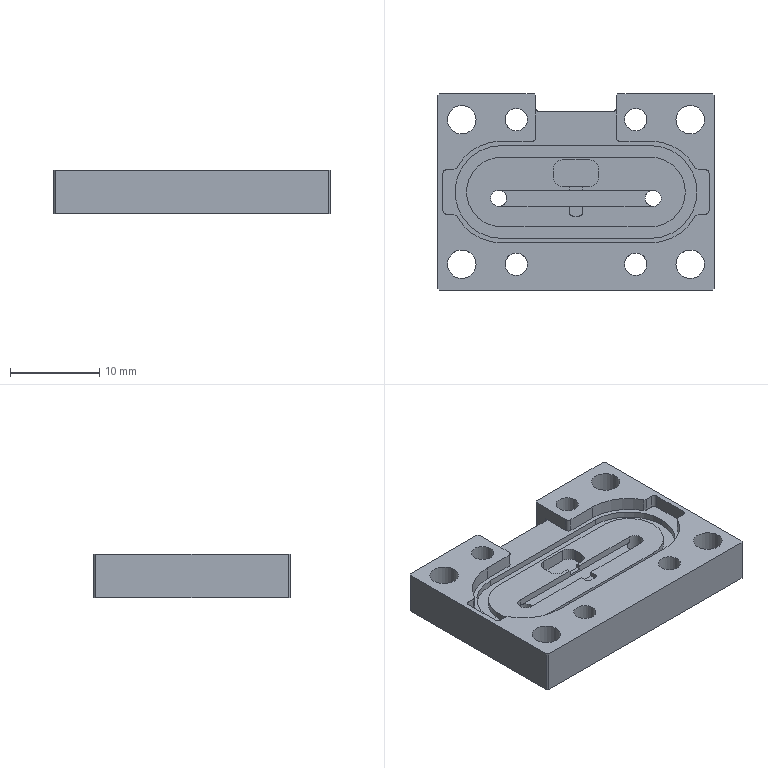NC program | NX | posted with a generic post | part box 31 x 22 x 4.9 mm
Lines 5425 to 7598 of 7945, first 1786 of 2168 lines:
(PLANAR_MILL_4_COPY_1 , TOOL : D0.8)
N10716 T10 M6
N10718 G54
N10720 G17 G0 G90 X-12.458 Y2.063 S3500 M3
N10722 G43 Z20. H10
N10724 Z0.14
N10726 G94 G1 Z-0.06 F200.
N10728 G41 X-12.493 Y2.157 D10
N10730 G3 X-13.18 Y2.327 R0.5
N10732 G1 X-13.463 Y2.157
N10734 G2 X-13.669 Y2.1 R0.4
N10736 G1 X-14.5
N10738 Y-2.1
N10740 X-13.669
N10742 G2 X-13.463 Y-2.157 R0.4
N10744 G1 X-13.18 Y-2.327
N10746 G3 X-12.493 Y-2.157 R0.5
N10748 G40
N10750 G1 X-12.458 Y-2.063
N10752 Z0.14
N10754 G0 Y2.063 Z0.08
N10756 G1 Z-0.12
N10758 G41 X-12.493 Y2.157
N10760 G3 X-13.18 Y2.327 R0.5
N10762 G1 X-13.463 Y2.157
N10764 G2 X-13.669 Y2.1 R0.4
N10766 G1 X-14.5
N10768 Y-2.1
N10770 X-13.669
N10772 G2 X-13.463 Y-2.157 R0.4
N10774 G1 X-13.18 Y-2.327
N10776 G3 X-12.493 Y-2.157 R0.5
N10778 G40
N10780 G1 X-12.458 Y-2.063
N10782 Z0.08
N10784 G0 Y2.063 Z0.02
N10786 G1 Z-0.18
N10788 G41 X-12.493 Y2.157
N10790 G3 X-13.18 Y2.327 R0.5
N10792 G1 X-13.463 Y2.157
N10794 G2 X-13.669 Y2.1 R0.4
N10796 G1 X-14.5
N10798 Y-2.1
N10800 X-13.669
N10802 G2 X-13.463 Y-2.157 R0.4
N10804 G1 X-13.18 Y-2.327
N10806 G3 X-12.493 Y-2.157 R0.5
N10808 G40
N10810 G1 X-12.458 Y-2.063
N10812 Z0.02
N10814 G0 Y2.063 Z-0.04
N10816 G1 Z-0.24
N10818 G41 X-12.493 Y2.157
N10820 G3 X-13.18 Y2.327 R0.5
N10822 G1 X-13.463 Y2.157
N10824 G2 X-13.669 Y2.1 R0.4
N10826 G1 X-14.5
N10828 Y-2.1
N10830 X-13.669
N10832 G2 X-13.463 Y-2.157 R0.4
N10834 G1 X-13.18 Y-2.327
N10836 G3 X-12.493 Y-2.157 R0.5
N10838 G40
N10840 G1 X-12.458 Y-2.063
N10842 Z-0.04
N10844 G0 Y2.063 Z-0.1
N10846 G1 Z-0.3
N10848 G41 X-12.493 Y2.157
N10850 G3 X-13.18 Y2.327 R0.5
N10852 G1 X-13.463 Y2.157
N10854 G2 X-13.669 Y2.1 R0.4
N10856 G1 X-14.5
N10858 Y-2.1
N10860 X-13.669
N10862 G2 X-13.463 Y-2.157 R0.4
N10864 G1 X-13.18 Y-2.327
N10866 G3 X-12.493 Y-2.157 R0.5
N10868 G40
N10870 G1 X-12.458 Y-2.063
N10872 Z-0.1
N10874 G0 Y2.063 Z-0.16
N10876 G1 Z-0.36
N10878 G41 X-12.493 Y2.157
N10880 G3 X-13.18 Y2.327 R0.5
N10882 G1 X-13.463 Y2.157
N10884 G2 X-13.669 Y2.1 R0.4
N10886 G1 X-14.5
N10888 Y-2.1
N10890 X-13.669
N10892 G2 X-13.463 Y-2.157 R0.4
N10894 G1 X-13.18 Y-2.327
N10896 G3 X-12.493 Y-2.157 R0.5
N10898 G40
N10900 G1 X-12.458 Y-2.063
N10902 Z-0.16
N10904 G0 Y2.063 Z-0.22
N10906 G1 Z-0.42
N10908 G41 X-12.493 Y2.157
N10910 G3 X-13.18 Y2.327 R0.5
N10912 G1 X-13.463 Y2.157
N10914 G2 X-13.669 Y2.1 R0.4
N10916 G1 X-14.5
N10918 Y-2.1
N10920 X-13.669
N10922 G2 X-13.463 Y-2.157 R0.4
N10924 G1 X-13.18 Y-2.327
N10926 G3 X-12.493 Y-2.157 R0.5
N10928 G40
N10930 G1 X-12.458 Y-2.063
N10932 Z-0.22
N10934 G0 Y2.063 Z-0.28
N10936 G1 Z-0.48
N10938 G41 X-12.493 Y2.157
N10940 G3 X-13.18 Y2.327 R0.5
N10942 G1 X-13.463 Y2.157
N10944 G2 X-13.669 Y2.1 R0.4
N10946 G1 X-14.5
N10948 Y-2.1
N10950 X-13.669
N10952 G2 X-13.463 Y-2.157 R0.4
N10954 G1 X-13.18 Y-2.327
N10956 G3 X-12.493 Y-2.157 R0.5
N10958 G40
N10960 G1 X-12.458 Y-2.063
N10962 Z-0.28
N10964 G0 Y2.063 Z-0.34
N10966 G1 Z-0.54
N10968 G41 X-12.493 Y2.157
N10970 G3 X-13.18 Y2.327 R0.5
N10972 G1 X-13.463 Y2.157
N10974 G2 X-13.669 Y2.1 R0.4
N10976 G1 X-14.5
N10978 Y-2.1
N10980 X-13.669
N10982 G2 X-13.463 Y-2.157 R0.4
N10984 G1 X-13.18 Y-2.327
N10986 G3 X-12.493 Y-2.157 R0.5
N10988 G40
N10990 G1 X-12.458 Y-2.063
N10992 Z-0.34
N10994 G0 Y2.063 Z-0.4
N10996 G1 Z-0.6
N10998 G41 X-12.493 Y2.157
N11000 G3 X-13.18 Y2.327 R0.5
N11002 G1 X-13.463 Y2.157
N11004 G2 X-13.669 Y2.1 R0.4
N11006 G1 X-14.5
N11008 Y-2.1
N11010 X-13.669
N11012 G2 X-13.463 Y-2.157 R0.4
N11014 G1 X-13.18 Y-2.327
N11016 G3 X-12.493 Y-2.157 R0.5
N11018 G40
N11020 G1 X-12.458 Y-2.063
N11022 Z-0.4
N11024 G0 Y2.063 Z-0.46
N11026 G1 Z-0.66
N11028 G41 X-12.493 Y2.157
N11030 G3 X-13.18 Y2.327 R0.5
N11032 G1 X-13.463 Y2.157
N11034 G2 X-13.669 Y2.1 R0.4
N11036 G1 X-14.5
N11038 Y-2.1
N11040 X-13.669
N11042 G2 X-13.463 Y-2.157 R0.4
N11044 G1 X-13.18 Y-2.327
N11046 G3 X-12.493 Y-2.157 R0.5
N11048 G40
N11050 G1 X-12.458 Y-2.063
N11052 Z-0.46
N11054 G0 Y2.063 Z-0.52
N11056 G1 Z-0.72
N11058 G41 X-12.493 Y2.157
N11060 G3 X-13.18 Y2.327 R0.5
N11062 G1 X-13.463 Y2.157
N11064 G2 X-13.669 Y2.1 R0.4
N11066 G1 X-14.5
N11068 Y-2.1
N11070 X-13.669
N11072 G2 X-13.463 Y-2.157 R0.4
N11074 G1 X-13.18 Y-2.327
N11076 G3 X-12.493 Y-2.157 R0.5
N11078 G40
N11080 G1 X-12.458 Y-2.063
N11082 Z-0.52
N11084 G0 Y2.063 Z-0.58
N11086 G1 Z-0.78
N11088 G41 X-12.493 Y2.157
N11090 G3 X-13.18 Y2.327 R0.5
N11092 G1 X-13.463 Y2.157
N11094 G2 X-13.669 Y2.1 R0.4
N11096 G1 X-14.5
N11098 Y-2.1
N11100 X-13.669
N11102 G2 X-13.463 Y-2.157 R0.4
N11104 G1 X-13.18 Y-2.327
N11106 G3 X-12.493 Y-2.157 R0.5
N11108 G40
N11110 G1 X-12.458 Y-2.063
N11112 Z-0.58
N11114 G0 Y2.063 Z-0.64
N11116 G1 Z-0.84
N11118 G41 X-12.493 Y2.157
N11120 G3 X-13.18 Y2.327 R0.5
N11122 G1 X-13.463 Y2.157
N11124 G2 X-13.669 Y2.1 R0.4
N11126 G1 X-14.5
N11128 Y-2.1
N11130 X-13.669
N11132 G2 X-13.463 Y-2.157 R0.4
N11134 G1 X-13.18 Y-2.327
N11136 G3 X-12.493 Y-2.157 R0.5
N11138 G40
N11140 G1 X-12.458 Y-2.063
N11142 Z-0.64
N11144 G0 Y2.063 Z-0.7
N11146 G1 Z-0.9
N11148 G41 X-12.493 Y2.157
N11150 G3 X-13.18 Y2.327 R0.5
N11152 G1 X-13.463 Y2.157
N11154 G2 X-13.669 Y2.1 R0.4
N11156 G1 X-14.5
N11158 Y-2.1
N11160 X-13.669
N11162 G2 X-13.463 Y-2.157 R0.4
N11164 G1 X-13.18 Y-2.327
N11166 G3 X-12.493 Y-2.157 R0.5
N11168 G40
N11170 G1 X-12.458 Y-2.063
N11172 Z-0.7
N11174 G0 Y2.063 Z-0.76
N11176 G1 Z-0.96
N11178 G41 X-12.493 Y2.157
N11180 G3 X-13.18 Y2.327 R0.5
N11182 G1 X-13.463 Y2.157
N11184 G2 X-13.669 Y2.1 R0.4
N11186 G1 X-14.5
N11188 Y-2.1
N11190 X-13.669
N11192 G2 X-13.463 Y-2.157 R0.4
N11194 G1 X-13.18 Y-2.327
N11196 G3 X-12.493 Y-2.157 R0.5
N11198 G40
N11200 G1 X-12.458 Y-2.063
N11202 Z-0.76
N11204 G0 Y2.063 Z-0.82
N11206 G1 Z-1.02
N11208 G41 X-12.493 Y2.157
N11210 G3 X-13.18 Y2.327 R0.5
N11212 G1 X-13.463 Y2.157
N11214 G2 X-13.669 Y2.1 R0.4
N11216 G1 X-14.5
N11218 Y-2.1
N11220 X-13.669
N11222 G2 X-13.463 Y-2.157 R0.4
N11224 G1 X-13.18 Y-2.327
N11226 G3 X-12.493 Y-2.157 R0.5
N11228 G40
N11230 G1 X-12.458 Y-2.063
N11232 Z-0.82
N11234 G0 Y2.063 Z-0.88
N11236 G1 Z-1.08
N11238 G41 X-12.493 Y2.157
N11240 G3 X-13.18 Y2.327 R0.5
N11242 G1 X-13.463 Y2.157
N11244 G2 X-13.669 Y2.1 R0.4
N11246 G1 X-14.5
N11248 Y-2.1
N11250 X-13.669
N11252 G2 X-13.463 Y-2.157 R0.4
N11254 G1 X-13.18 Y-2.327
N11256 G3 X-12.493 Y-2.157 R0.5
N11258 G40
N11260 G1 X-12.458 Y-2.063
N11262 Z-0.88
N11264 G0 Y2.063 Z-0.94
N11266 G1 Z-1.14
N11268 G41 X-12.493 Y2.157
N11270 G3 X-13.18 Y2.327 R0.5
N11272 G1 X-13.463 Y2.157
N11274 G2 X-13.669 Y2.1 R0.4
N11276 G1 X-14.5
N11278 Y-2.1
N11280 X-13.669
N11282 G2 X-13.463 Y-2.157 R0.4
N11284 G1 X-13.18 Y-2.327
N11286 G3 X-12.493 Y-2.157 R0.5
N11288 G40
N11290 G1 X-12.458 Y-2.063
N11292 Z-0.94
N11294 G0 Y2.063 Z-1.
N11296 G1 Z-1.2
N11298 G41 X-12.493 Y2.157
N11300 G3 X-13.18 Y2.327 R0.5
N11302 G1 X-13.463 Y2.157
N11304 G2 X-13.669 Y2.1 R0.4
N11306 G1 X-14.5
N11308 Y-2.1
N11310 X-13.669
N11312 G2 X-13.463 Y-2.157 R0.4
N11314 G1 X-13.18 Y-2.327
N11316 G3 X-12.493 Y-2.157 R0.5
N11318 G40
N11320 G1 X-12.458 Y-2.063
N11322 Z-1.
N11324 G0 Y2.063 Z-1.06
N11326 G1 Z-1.26
N11328 G41 X-12.493 Y2.157
N11330 G3 X-13.18 Y2.327 R0.5
N11332 G1 X-13.463 Y2.157
N11334 G2 X-13.669 Y2.1 R0.4
N11336 G1 X-14.5
N11338 Y-2.1
N11340 X-13.669
N11342 G2 X-13.463 Y-2.157 R0.4
N11344 G1 X-13.18 Y-2.327
N11346 G3 X-12.493 Y-2.157 R0.5
N11348 G40
N11350 G1 X-12.458 Y-2.063
N11352 Z-1.06
N11354 G0 Y2.063 Z-1.12
N11356 G1 Z-1.32
N11358 G41 X-12.493 Y2.157
N11360 G3 X-13.18 Y2.327 R0.5
N11362 G1 X-13.463 Y2.157
N11364 G2 X-13.669 Y2.1 R0.4
N11366 G1 X-14.5
N11368 Y-2.1
N11370 X-13.669
N11372 G2 X-13.463 Y-2.157 R0.4
N11374 G1 X-13.18 Y-2.327
N11376 G3 X-12.493 Y-2.157 R0.5
N11378 G40
N11380 G1 X-12.458 Y-2.063
N11382 Z-1.12
N11384 G0 Y2.063 Z-1.18
N11386 G1 Z-1.38
N11388 G41 X-12.493 Y2.157
N11390 G3 X-13.18 Y2.327 R0.5
N11392 G1 X-13.463 Y2.157
N11394 G2 X-13.669 Y2.1 R0.4
N11396 G1 X-14.5
N11398 Y-2.1
N11400 X-13.669
N11402 G2 X-13.463 Y-2.157 R0.4
N11404 G1 X-13.18 Y-2.327
N11406 G3 X-12.493 Y-2.157 R0.5
N11408 G40
N11410 G1 X-12.458 Y-2.063
N11412 Z-1.18
N11414 G0 Y2.063 Z-1.24
N11416 G1 Z-1.44
N11418 G41 X-12.493 Y2.157
N11420 G3 X-13.18 Y2.327 R0.5
N11422 G1 X-13.463 Y2.157
N11424 G2 X-13.669 Y2.1 R0.4
N11426 G1 X-14.5
N11428 Y-2.1
N11430 X-13.669
N11432 G2 X-13.463 Y-2.157 R0.4
N11434 G1 X-13.18 Y-2.327
N11436 G3 X-12.493 Y-2.157 R0.5
N11438 G40
N11440 G1 X-12.458 Y-2.063
N11442 Z-1.24
N11444 G0 Y2.063 Z-1.3
N11446 G1 Z-1.5
N11448 G41 X-12.493 Y2.157
N11450 G3 X-13.18 Y2.327 R0.5
N11452 G1 X-13.463 Y2.157
N11454 G2 X-13.669 Y2.1 R0.4
N11456 G1 X-14.5
N11458 Y-2.1
N11460 X-13.669
N11462 G2 X-13.463 Y-2.157 R0.4
N11464 G1 X-13.18 Y-2.327
N11466 G3 X-12.493 Y-2.157 R0.5
N11468 G40
N11470 G1 X-12.458 Y-2.063
N11472 Z-1.3
N11474 G0 Z3.
N11476 X12.458
N11478 Z0.14
N11480 G1 Z-0.06
N11482 G41 X12.493 Y-2.157
N11484 G3 X13.18 Y-2.327 R0.5
N11486 G1 X13.463 Y-2.157
N11488 G2 X13.669 Y-2.1 R0.4
N11490 G1 X14.5
N11492 Y2.1
N11494 X13.669
N11496 G2 X13.463 Y2.157 R0.4
N11498 G1 X13.18 Y2.327
N11500 G3 X12.493 Y2.157 R0.5
N11502 G40
N11504 G1 X12.458 Y2.063
N11506 Z0.14
N11508 G0 Y-2.063 Z0.08
N11510 G1 Z-0.12
N11512 G41 X12.493 Y-2.157
N11514 G3 X13.18 Y-2.327 R0.5
N11516 G1 X13.463 Y-2.157
N11518 G2 X13.669 Y-2.1 R0.4
N11520 G1 X14.5
N11522 Y2.1
N11524 X13.669
N11526 G2 X13.463 Y2.157 R0.4
N11528 G1 X13.18 Y2.327
N11530 G3 X12.493 Y2.157 R0.5
N11532 G40
N11534 G1 X12.458 Y2.063
N11536 Z0.08
N11538 G0 Y-2.063 Z0.02
N11540 G1 Z-0.18
N11542 G41 X12.493 Y-2.157
N11544 G3 X13.18 Y-2.327 R0.5
N11546 G1 X13.463 Y-2.157
N11548 G2 X13.669 Y-2.1 R0.4
N11550 G1 X14.5
N11552 Y2.1
N11554 X13.669
N11556 G2 X13.463 Y2.157 R0.4
N11558 G1 X13.18 Y2.327
N11560 G3 X12.493 Y2.157 R0.5
N11562 G40
N11564 G1 X12.458 Y2.063
N11566 Z0.02
N11568 G0 Y-2.063 Z-0.04
N11570 G1 Z-0.24
N11572 G41 X12.493 Y-2.157
N11574 G3 X13.18 Y-2.327 R0.5
N11576 G1 X13.463 Y-2.157
N11578 G2 X13.669 Y-2.1 R0.4
N11580 G1 X14.5
N11582 Y2.1
N11584 X13.669
N11586 G2 X13.463 Y2.157 R0.4
N11588 G1 X13.18 Y2.327
N11590 G3 X12.493 Y2.157 R0.5
N11592 G40
N11594 G1 X12.458 Y2.063
N11596 Z-0.04
N11598 G0 Y-2.063 Z-0.1
N11600 G1 Z-0.3
N11602 G41 X12.493 Y-2.157
N11604 G3 X13.18 Y-2.327 R0.5
N11606 G1 X13.463 Y-2.157
N11608 G2 X13.669 Y-2.1 R0.4
N11610 G1 X14.5
N11612 Y2.1
N11614 X13.669
N11616 G2 X13.463 Y2.157 R0.4
N11618 G1 X13.18 Y2.327
N11620 G3 X12.493 Y2.157 R0.5
N11622 G40
N11624 G1 X12.458 Y2.063
N11626 Z-0.1
N11628 G0 Y-2.063 Z-0.16
N11630 G1 Z-0.36
N11632 G41 X12.493 Y-2.157
N11634 G3 X13.18 Y-2.327 R0.5
N11636 G1 X13.463 Y-2.157
N11638 G2 X13.669 Y-2.1 R0.4
N11640 G1 X14.5
N11642 Y2.1
N11644 X13.669
N11646 G2 X13.463 Y2.157 R0.4
N11648 G1 X13.18 Y2.327
N11650 G3 X12.493 Y2.157 R0.5
N11652 G40
N11654 G1 X12.458 Y2.063
N11656 Z-0.16
N11658 G0 Y-2.063 Z-0.22
N11660 G1 Z-0.42
N11662 G41 X12.493 Y-2.157
N11664 G3 X13.18 Y-2.327 R0.5
N11666 G1 X13.463 Y-2.157
N11668 G2 X13.669 Y-2.1 R0.4
N11670 G1 X14.5
N11672 Y2.1
N11674 X13.669
N11676 G2 X13.463 Y2.157 R0.4
N11678 G1 X13.18 Y2.327
N11680 G3 X12.493 Y2.157 R0.5
N11682 G40
N11684 G1 X12.458 Y2.063
N11686 Z-0.22
N11688 G0 Y-2.063 Z-0.28
N11690 G1 Z-0.48
N11692 G41 X12.493 Y-2.157
N11694 G3 X13.18 Y-2.327 R0.5
N11696 G1 X13.463 Y-2.157
N11698 G2 X13.669 Y-2.1 R0.4
N11700 G1 X14.5
N11702 Y2.1
N11704 X13.669
N11706 G2 X13.463 Y2.157 R0.4
N11708 G1 X13.18 Y2.327
N11710 G3 X12.493 Y2.157 R0.5
N11712 G40
N11714 G1 X12.458 Y2.063
N11716 Z-0.28
N11718 G0 Y-2.063 Z-0.34
N11720 G1 Z-0.54
N11722 G41 X12.493 Y-2.157
N11724 G3 X13.18 Y-2.327 R0.5
N11726 G1 X13.463 Y-2.157
N11728 G2 X13.669 Y-2.1 R0.4
N11730 G1 X14.5
N11732 Y2.1
N11734 X13.669
N11736 G2 X13.463 Y2.157 R0.4
N11738 G1 X13.18 Y2.327
N11740 G3 X12.493 Y2.157 R0.5
N11742 G40
N11744 G1 X12.458 Y2.063
N11746 Z-0.34
N11748 G0 Y-2.063 Z-0.4
N11750 G1 Z-0.6
N11752 G41 X12.493 Y-2.157
N11754 G3 X13.18 Y-2.327 R0.5
N11756 G1 X13.463 Y-2.157
N11758 G2 X13.669 Y-2.1 R0.4
N11760 G1 X14.5
N11762 Y2.1
N11764 X13.669
N11766 G2 X13.463 Y2.157 R0.4
N11768 G1 X13.18 Y2.327
N11770 G3 X12.493 Y2.157 R0.5
N11772 G40
N11774 G1 X12.458 Y2.063
N11776 Z-0.4
N11778 G0 Y-2.063 Z-0.46
N11780 G1 Z-0.66
N11782 G41 X12.493 Y-2.157
N11784 G3 X13.18 Y-2.327 R0.5
N11786 G1 X13.463 Y-2.157
N11788 G2 X13.669 Y-2.1 R0.4
N11790 G1 X14.5
N11792 Y2.1
N11794 X13.669
N11796 G2 X13.463 Y2.157 R0.4
N11798 G1 X13.18 Y2.327
N11800 G3 X12.493 Y2.157 R0.5
N11802 G40
N11804 G1 X12.458 Y2.063
N11806 Z-0.46
N11808 G0 Y-2.063 Z-0.52
N11810 G1 Z-0.72
N11812 G41 X12.493 Y-2.157
N11814 G3 X13.18 Y-2.327 R0.5
N11816 G1 X13.463 Y-2.157
N11818 G2 X13.669 Y-2.1 R0.4
N11820 G1 X14.5
N11822 Y2.1
N11824 X13.669
N11826 G2 X13.463 Y2.157 R0.4
N11828 G1 X13.18 Y2.327
N11830 G3 X12.493 Y2.157 R0.5
N11832 G40
N11834 G1 X12.458 Y2.063
N11836 Z-0.52
N11838 G0 Y-2.063 Z-0.58
N11840 G1 Z-0.78
N11842 G41 X12.493 Y-2.157
N11844 G3 X13.18 Y-2.327 R0.5
N11846 G1 X13.463 Y-2.157
N11848 G2 X13.669 Y-2.1 R0.4
N11850 G1 X14.5
N11852 Y2.1
N11854 X13.669
N11856 G2 X13.463 Y2.157 R0.4
N11858 G1 X13.18 Y2.327
N11860 G3 X12.493 Y2.157 R0.5
N11862 G40
N11864 G1 X12.458 Y2.063
N11866 Z-0.58
N11868 G0 Y-2.063 Z-0.64
N11870 G1 Z-0.84
N11872 G41 X12.493 Y-2.157
N11874 G3 X13.18 Y-2.327 R0.5
N11876 G1 X13.463 Y-2.157
N11878 G2 X13.669 Y-2.1 R0.4
N11880 G1 X14.5
N11882 Y2.1
N11884 X13.669
N11886 G2 X13.463 Y2.157 R0.4
N11888 G1 X13.18 Y2.327
N11890 G3 X12.493 Y2.157 R0.5
N11892 G40
N11894 G1 X12.458 Y2.063
N11896 Z-0.64
N11898 G0 Y-2.063 Z-0.7
N11900 G1 Z-0.9
N11902 G41 X12.493 Y-2.157
N11904 G3 X13.18 Y-2.327 R0.5
N11906 G1 X13.463 Y-2.157
N11908 G2 X13.669 Y-2.1 R0.4
N11910 G1 X14.5
N11912 Y2.1
N11914 X13.669
N11916 G2 X13.463 Y2.157 R0.4
N11918 G1 X13.18 Y2.327
N11920 G3 X12.493 Y2.157 R0.5
N11922 G40
N11924 G1 X12.458 Y2.063
N11926 Z-0.7
N11928 G0 Y-2.063 Z-0.76
N11930 G1 Z-0.96
N11932 G41 X12.493 Y-2.157
N11934 G3 X13.18 Y-2.327 R0.5
N11936 G1 X13.463 Y-2.157
N11938 G2 X13.669 Y-2.1 R0.4
N11940 G1 X14.5
N11942 Y2.1
N11944 X13.669
N11946 G2 X13.463 Y2.157 R0.4
N11948 G1 X13.18 Y2.327
N11950 G3 X12.493 Y2.157 R0.5
N11952 G40
N11954 G1 X12.458 Y2.063
N11956 Z-0.76
N11958 G0 Y-2.063 Z-0.82
N11960 G1 Z-1.02
N11962 G41 X12.493 Y-2.157
N11964 G3 X13.18 Y-2.327 R0.5
N11966 G1 X13.463 Y-2.157
N11968 G2 X13.669 Y-2.1 R0.4
N11970 G1 X14.5
N11972 Y2.1
N11974 X13.669
N11976 G2 X13.463 Y2.157 R0.4
N11978 G1 X13.18 Y2.327
N11980 G3 X12.493 Y2.157 R0.5
N11982 G40
N11984 G1 X12.458 Y2.063
N11986 Z-0.82
N11988 G0 Y-2.063 Z-0.88
N11990 G1 Z-1.08
N11992 G41 X12.493 Y-2.157
N11994 G3 X13.18 Y-2.327 R0.5
N11996 G1 X13.463 Y-2.157
N11998 G2 X13.669 Y-2.1 R0.4
N12000 G1 X14.5
N12002 Y2.1
N12004 X13.669
N12006 G2 X13.463 Y2.157 R0.4
N12008 G1 X13.18 Y2.327
N12010 G3 X12.493 Y2.157 R0.5
N12012 G40
N12014 G1 X12.458 Y2.063
N12016 Z-0.88
N12018 G0 Y-2.063 Z-0.94
N12020 G1 Z-1.14
N12022 G41 X12.493 Y-2.157
N12024 G3 X13.18 Y-2.327 R0.5
N12026 G1 X13.463 Y-2.157
N12028 G2 X13.669 Y-2.1 R0.4
N12030 G1 X14.5
N12032 Y2.1
N12034 X13.669
N12036 G2 X13.463 Y2.157 R0.4
N12038 G1 X13.18 Y2.327
N12040 G3 X12.493 Y2.157 R0.5
N12042 G40
N12044 G1 X12.458 Y2.063
N12046 Z-0.94
N12048 G0 Y-2.063 Z-1.
N12050 G1 Z-1.2
N12052 G41 X12.493 Y-2.157
N12054 G3 X13.18 Y-2.327 R0.5
N12056 G1 X13.463 Y-2.157
N12058 G2 X13.669 Y-2.1 R0.4
N12060 G1 X14.5
N12062 Y2.1
N12064 X13.669
N12066 G2 X13.463 Y2.157 R0.4
N12068 G1 X13.18 Y2.327
N12070 G3 X12.493 Y2.157 R0.5
N12072 G40
N12074 G1 X12.458 Y2.063
N12076 Z-1.
N12078 G0 Y-2.063 Z-1.06
N12080 G1 Z-1.26
N12082 G41 X12.493 Y-2.157
N12084 G3 X13.18 Y-2.327 R0.5
N12086 G1 X13.463 Y-2.157
N12088 G2 X13.669 Y-2.1 R0.4
N12090 G1 X14.5
N12092 Y2.1
N12094 X13.669
N12096 G2 X13.463 Y2.157 R0.4
N12098 G1 X13.18 Y2.327
N12100 G3 X12.493 Y2.157 R0.5
N12102 G40
N12104 G1 X12.458 Y2.063
N12106 Z-1.06
N12108 G0 Y-2.063 Z-1.12
N12110 G1 Z-1.32
N12112 G41 X12.493 Y-2.157
N12114 G3 X13.18 Y-2.327 R0.5
N12116 G1 X13.463 Y-2.157
N12118 G2 X13.669 Y-2.1 R0.4
N12120 G1 X14.5
N12122 Y2.1
N12124 X13.669
N12126 G2 X13.463 Y2.157 R0.4
N12128 G1 X13.18 Y2.327
N12130 G3 X12.493 Y2.157 R0.5
N12132 G40
N12134 G1 X12.458 Y2.063
N12136 Z-1.12
N12138 G0 Y-2.063 Z-1.18
N12140 G1 Z-1.38
N12142 G41 X12.493 Y-2.157
N12144 G3 X13.18 Y-2.327 R0.5
N12146 G1 X13.463 Y-2.157
N12148 G2 X13.669 Y-2.1 R0.4
N12150 G1 X14.5
N12152 Y2.1
N12154 X13.669
N12156 G2 X13.463 Y2.157 R0.4
N12158 G1 X13.18 Y2.327
N12160 G3 X12.493 Y2.157 R0.5
N12162 G40
N12164 G1 X12.458 Y2.063
N12166 Z-1.18
N12168 G0 Y-2.063 Z-1.24
N12170 G1 Z-1.44
N12172 G41 X12.493 Y-2.157
N12174 G3 X13.18 Y-2.327 R0.5
N12176 G1 X13.463 Y-2.157
N12178 G2 X13.669 Y-2.1 R0.4
N12180 G1 X14.5
N12182 Y2.1
N12184 X13.669
N12186 G2 X13.463 Y2.157 R0.4
N12188 G1 X13.18 Y2.327
N12190 G3 X12.493 Y2.157 R0.5
N12192 G40
N12194 G1 X12.458 Y2.063
N12196 Z-1.24
N12198 G0 Y-2.063 Z-1.3
N12200 G1 Z-1.5
N12202 G41 X12.493 Y-2.157
N12204 G3 X13.18 Y-2.327 R0.5
N12206 G1 X13.463 Y-2.157
N12208 G2 X13.669 Y-2.1 R0.4
N12210 G1 X14.5
N12212 Y2.1
N12214 X13.669
N12216 G2 X13.463 Y2.157 R0.4
N12218 G1 X13.18 Y2.327
N12220 G3 X12.493 Y2.157 R0.5
N12222 G40
N12224 G1 X12.458 Y2.063
N12226 Z-1.3
N12228 G0 Z20.
(PLANAR_MILL_4_COPY_COPY , TOOL : D0.8)
N12230 X-4.335 Y12.047
N12232 Z0.14
N12234 G1 Z-0.06
N12236 G41 X-4.417 Y11.99
N12238 G3 X-4.417 Y11.283 R0.5
N12240 G1 X-4.217 Y11.083
N12242 G2 X-4.1 Y10.8 R0.4
N12244 G1 Y9.4
N12246 X4.1
N12248 Y10.8
N12250 G2 X4.217 Y11.083 R0.4
N12252 G1 X4.417 Y11.283
N12254 G3 X4.417 Y11.99 R0.5
N12256 G40
N12258 G1 X4.335 Y12.047
N12260 Z0.14
N12262 G0 X-4.335 Z0.08
N12264 G1 Z-0.12
N12266 G41 X-4.417 Y11.99
N12268 G3 X-4.417 Y11.283 R0.5
N12270 G1 X-4.217 Y11.083
N12272 G2 X-4.1 Y10.8 R0.4
N12274 G1 Y9.4
N12276 X4.1
N12278 Y10.8
N12280 G2 X4.217 Y11.083 R0.4
N12282 G1 X4.417 Y11.283
N12284 G3 X4.417 Y11.99 R0.5
N12286 G40
N12288 G1 X4.335 Y12.047
N12290 Z0.08
N12292 G0 X-4.335 Z0.02
N12294 G1 Z-0.18
N12296 G41 X-4.417 Y11.99
N12298 G3 X-4.417 Y11.283 R0.5
N12300 G1 X-4.217 Y11.083
N12302 G2 X-4.1 Y10.8 R0.4
N12304 G1 Y9.4
N12306 X4.1
N12308 Y10.8
N12310 G2 X4.217 Y11.083 R0.4
N12312 G1 X4.417 Y11.283
N12314 G3 X4.417 Y11.99 R0.5
N12316 G40
N12318 G1 X4.335 Y12.047
N12320 Z0.02
N12322 G0 X-4.335 Z-0.04
N12324 G1 Z-0.24
N12326 G41 X-4.417 Y11.99
N12328 G3 X-4.417 Y11.283 R0.5
N12330 G1 X-4.217 Y11.083
N12332 G2 X-4.1 Y10.8 R0.4
N12334 G1 Y9.4
N12336 X4.1
N12338 Y10.8
N12340 G2 X4.217 Y11.083 R0.4
N12342 G1 X4.417 Y11.283
N12344 G3 X4.417 Y11.99 R0.5
N12346 G40
N12348 G1 X4.335 Y12.047
N12350 Z-0.04
N12352 G0 X-4.335 Z-0.1
N12354 G1 Z-0.3
N12356 G41 X-4.417 Y11.99
N12358 G3 X-4.417 Y11.283 R0.5
N12360 G1 X-4.217 Y11.083
N12362 G2 X-4.1 Y10.8 R0.4
N12364 G1 Y9.4
N12366 X4.1
N12368 Y10.8
N12370 G2 X4.217 Y11.083 R0.4
N12372 G1 X4.417 Y11.283
N12374 G3 X4.417 Y11.99 R0.5
N12376 G40
N12378 G1 X4.335 Y12.047
N12380 Z-0.1
N12382 G0 X-4.335 Z-0.16
N12384 G1 Z-0.36
N12386 G41 X-4.417 Y11.99
N12388 G3 X-4.417 Y11.283 R0.5
N12390 G1 X-4.217 Y11.083
N12392 G2 X-4.1 Y10.8 R0.4
N12394 G1 Y9.4
N12396 X4.1
N12398 Y10.8
N12400 G2 X4.217 Y11.083 R0.4
N12402 G1 X4.417 Y11.283
N12404 G3 X4.417 Y11.99 R0.5
N12406 G40
N12408 G1 X4.335 Y12.047
N12410 Z-0.16
N12412 G0 X-4.335 Z-0.22
N12414 G1 Z-0.42
N12416 G41 X-4.417 Y11.99
N12418 G3 X-4.417 Y11.283 R0.5
N12420 G1 X-4.217 Y11.083
N12422 G2 X-4.1 Y10.8 R0.4
N12424 G1 Y9.4
N12426 X4.1
N12428 Y10.8
N12430 G2 X4.217 Y11.083 R0.4
N12432 G1 X4.417 Y11.283
N12434 G3 X4.417 Y11.99 R0.5
N12436 G40
N12438 G1 X4.335 Y12.047
N12440 Z-0.22
N12442 G0 X-4.335 Z-0.28
N12444 G1 Z-0.48
N12446 G41 X-4.417 Y11.99
N12448 G3 X-4.417 Y11.283 R0.5
N12450 G1 X-4.217 Y11.083
N12452 G2 X-4.1 Y10.8 R0.4
N12454 G1 Y9.4
N12456 X4.1
N12458 Y10.8
N12460 G2 X4.217 Y11.083 R0.4
N12462 G1 X4.417 Y11.283
N12464 G3 X4.417 Y11.99 R0.5
N12466 G40
N12468 G1 X4.335 Y12.047
N12470 Z-0.28
N12472 G0 X-4.335 Z-0.34
N12474 G1 Z-0.54
N12476 G41 X-4.417 Y11.99
N12478 G3 X-4.417 Y11.283 R0.5
N12480 G1 X-4.217 Y11.083
N12482 G2 X-4.1 Y10.8 R0.4
N12484 G1 Y9.4
N12486 X4.1
N12488 Y10.8
N12490 G2 X4.217 Y11.083 R0.4
N12492 G1 X4.417 Y11.283
N12494 G3 X4.417 Y11.99 R0.5
N12496 G40
N12498 G1 X4.335 Y12.047
N12500 Z-0.34
N12502 G0 X-4.335 Z-0.4
N12504 G1 Z-0.6
N12506 G41 X-4.417 Y11.99
N12508 G3 X-4.417 Y11.283 R0.5
N12510 G1 X-4.217 Y11.083
N12512 G2 X-4.1 Y10.8 R0.4
N12514 G1 Y9.4
N12516 X4.1
N12518 Y10.8
N12520 G2 X4.217 Y11.083 R0.4
N12522 G1 X4.417 Y11.283
N12524 G3 X4.417 Y11.99 R0.5
N12526 G40
N12528 G1 X4.335 Y12.047
N12530 Z-0.4
N12532 G0 X-4.335 Z-0.46
N12534 G1 Z-0.66
N12536 G41 X-4.417 Y11.99
N12538 G3 X-4.417 Y11.283 R0.5
N12540 G1 X-4.217 Y11.083
N12542 G2 X-4.1 Y10.8 R0.4
N12544 G1 Y9.4
N12546 X4.1
N12548 Y10.8
N12550 G2 X4.217 Y11.083 R0.4
N12552 G1 X4.417 Y11.283
N12554 G3 X4.417 Y11.99 R0.5
N12556 G40
N12558 G1 X4.335 Y12.047
N12560 Z-0.46
N12562 G0 X-4.335 Z-0.52
N12564 G1 Z-0.72
N12566 G41 X-4.417 Y11.99
N12568 G3 X-4.417 Y11.283 R0.5
N12570 G1 X-4.217 Y11.083
N12572 G2 X-4.1 Y10.8 R0.4
N12574 G1 Y9.4
N12576 X4.1
N12578 Y10.8
N12580 G2 X4.217 Y11.083 R0.4
N12582 G1 X4.417 Y11.283
N12584 G3 X4.417 Y11.99 R0.5
N12586 G40
N12588 G1 X4.335 Y12.047
N12590 Z-0.52
N12592 G0 X-4.335 Z-0.58
N12594 G1 Z-0.78
N12596 G41 X-4.417 Y11.99
N12598 G3 X-4.417 Y11.283 R0.5
N12600 G1 X-4.217 Y11.083
N12602 G2 X-4.1 Y10.8 R0.4
N12604 G1 Y9.4
N12606 X4.1
N12608 Y10.8
N12610 G2 X4.217 Y11.083 R0.4
N12612 G1 X4.417 Y11.283
N12614 G3 X4.417 Y11.99 R0.5
N12616 G40
N12618 G1 X4.335 Y12.047
N12620 Z-0.58
N12622 G0 X-4.335 Z-0.64
N12624 G1 Z-0.84
N12626 G41 X-4.417 Y11.99
N12628 G3 X-4.417 Y11.283 R0.5
N12630 G1 X-4.217 Y11.083
N12632 G2 X-4.1 Y10.8 R0.4
N12634 G1 Y9.4
N12636 X4.1
N12638 Y10.8
N12640 G2 X4.217 Y11.083 R0.4
N12642 G1 X4.417 Y11.283
N12644 G3 X4.417 Y11.99 R0.5
N12646 G40
N12648 G1 X4.335 Y12.047
N12650 Z-0.64
N12652 G0 X-4.335 Z-0.7
N12654 G1 Z-0.9
N12656 G41 X-4.417 Y11.99
N12658 G3 X-4.417 Y11.283 R0.5
N12660 G1 X-4.217 Y11.083
N12662 G2 X-4.1 Y10.8 R0.4
N12664 G1 Y9.4
N12666 X4.1
N12668 Y10.8
N12670 G2 X4.217 Y11.083 R0.4
N12672 G1 X4.417 Y11.283
N12674 G3 X4.417 Y11.99 R0.5
N12676 G40
N12678 G1 X4.335 Y12.047
N12680 Z-0.7
N12682 G0 X-4.335 Z-0.76
N12684 G1 Z-0.96
N12686 G41 X-4.417 Y11.99
N12688 G3 X-4.417 Y11.283 R0.5
N12690 G1 X-4.217 Y11.083
N12692 G2 X-4.1 Y10.8 R0.4
N12694 G1 Y9.4
N12696 X4.1
N12698 Y10.8
N12700 G2 X4.217 Y11.083 R0.4
N12702 G1 X4.417 Y11.283
N12704 G3 X4.417 Y11.99 R0.5
N12706 G40
N12708 G1 X4.335 Y12.047
N12710 Z-0.76
N12712 G0 X-4.335 Z-0.82
N12714 G1 Z-1.02
N12716 G41 X-4.417 Y11.99
N12718 G3 X-4.417 Y11.283 R0.5
N12720 G1 X-4.217 Y11.083
N12722 G2 X-4.1 Y10.8 R0.4
N12724 G1 Y9.4
N12726 X4.1
N12728 Y10.8
N12730 G2 X4.217 Y11.083 R0.4
N12732 G1 X4.417 Y11.283
N12734 G3 X4.417 Y11.99 R0.5
N12736 G40
N12738 G1 X4.335 Y12.047
N12740 Z-0.82
N12742 G0 X-4.335 Z-0.88
N12744 G1 Z-1.08
N12746 G41 X-4.417 Y11.99
N12748 G3 X-4.417 Y11.283 R0.5
N12750 G1 X-4.217 Y11.083
N12752 G2 X-4.1 Y10.8 R0.4
N12754 G1 Y9.4
N12756 X4.1
N12758 Y10.8
N12760 G2 X4.217 Y11.083 R0.4
N12762 G1 X4.417 Y11.283
N12764 G3 X4.417 Y11.99 R0.5
N12766 G40
N12768 G1 X4.335 Y12.047
N12770 Z-0.88
N12772 G0 X-4.335 Z-0.94
N12774 G1 Z-1.14
N12776 G41 X-4.417 Y11.99
N12778 G3 X-4.417 Y11.283 R0.5
N12780 G1 X-4.217 Y11.083
N12782 G2 X-4.1 Y10.8 R0.4
N12784 G1 Y9.4
N12786 X4.1
N12788 Y10.8
N12790 G2 X4.217 Y11.083 R0.4
N12792 G1 X4.417 Y11.283
N12794 G3 X4.417 Y11.99 R0.5
N12796 G40
N12798 G1 X4.335 Y12.047
N12800 Z-0.94
N12802 G0 X-4.335 Z-1.
N12804 G1 Z-1.2
N12806 G41 X-4.417 Y11.99
N12808 G3 X-4.417 Y11.283 R0.5
N12810 G1 X-4.217 Y11.083
N12812 G2 X-4.1 Y10.8 R0.4
N12814 G1 Y9.4
N12816 X4.1
N12818 Y10.8
N12820 G2 X4.217 Y11.083 R0.4
N12822 G1 X4.417 Y11.283
N12824 G3 X4.417 Y11.99 R0.5
N12826 G40
N12828 G1 X4.335 Y12.047
N12830 Z-1.
N12832 G0 X-4.335 Z-1.06
N12834 G1 Z-1.26
N12836 G41 X-4.417 Y11.99
N12838 G3 X-4.417 Y11.283 R0.5
N12840 G1 X-4.217 Y11.083
N12842 G2 X-4.1 Y10.8 R0.4
N12844 G1 Y9.4
N12846 X4.1
N12848 Y10.8
N12850 G2 X4.217 Y11.083 R0.4
N12852 G1 X4.417 Y11.283
N12854 G3 X4.417 Y11.99 R0.5
N12856 G40
N12858 G1 X4.335 Y12.047
N12860 Z-1.06
N12862 G0 X-4.335 Z-1.12
N12864 G1 Z-1.32
N12866 G41 X-4.417 Y11.99
N12868 G3 X-4.417 Y11.283 R0.5
N12870 G1 X-4.217 Y11.083
N12872 G2 X-4.1 Y10.8 R0.4
N12874 G1 Y9.4
N12876 X4.1
N12878 Y10.8
N12880 G2 X4.217 Y11.083 R0.4
N12882 G1 X4.417 Y11.283
N12884 G3 X4.417 Y11.99 R0.5
N12886 G40
N12888 G1 X4.335 Y12.047
N12890 Z-1.12
N12892 G0 X-4.335 Z-1.18
N12894 G1 Z-1.38
N12896 G41 X-4.417 Y11.99
N12898 G3 X-4.417 Y11.283 R0.5
N12900 G1 X-4.217 Y11.083
N12902 G2 X-4.1 Y10.8 R0.4
N12904 G1 Y9.4
N12906 X4.1
N12908 Y10.8
N12910 G2 X4.217 Y11.083 R0.4
N12912 G1 X4.417 Y11.283
N12914 G3 X4.417 Y11.99 R0.5
N12916 G40
N12918 G1 X4.335 Y12.047
N12920 Z-1.18
N12922 G0 X-4.335 Z-1.24
N12924 G1 Z-1.44
N12926 G41 X-4.417 Y11.99
N12928 G3 X-4.417 Y11.283 R0.5
N12930 G1 X-4.217 Y11.083
N12932 G2 X-4.1 Y10.8 R0.4
N12934 G1 Y9.4
N12936 X4.1
N12938 Y10.8
N12940 G2 X4.217 Y11.083 R0.4
N12942 G1 X4.417 Y11.283
N12944 G3 X4.417 Y11.99 R0.5
N12946 G40
N12948 G1 X4.335 Y12.047
N12950 Z-1.24
N12952 G0 X-4.335 Z-1.3
N12954 G1 Z-1.5
N12956 G41 X-4.417 Y11.99
N12958 G3 X-4.417 Y11.283 R0.5
N12960 G1 X-4.217 Y11.083
N12962 G2 X-4.1 Y10.8 R0.4
N12964 G1 Y9.4
N12966 X4.1
N12968 Y10.8
N12970 G2 X4.217 Y11.083 R0.4
N12972 G1 X4.417 Y11.283
N12974 G3 X4.417 Y11.99 R0.5
N12976 G40
N12978 G1 X4.335 Y12.047
N12980 Z-1.3
N12982 G0 X-4.335 Z-1.36
N12984 G1 Z-1.56
N12986 G41 X-4.417 Y11.99
N12988 G3 X-4.417 Y11.283 R0.5
N12990 G1 X-4.217 Y11.083
N12992 G2 X-4.1 Y10.8 R0.4
N12994 G1 Y9.4
N12996 X4.1
N12998 Y10.8
N13000 G2 X4.217 Y11.083 R0.4
N13002 G1 X4.417 Y11.283
N13004 G3 X4.417 Y11.99 R0.5
N13006 G40
N13008 G1 X4.335 Y12.047
N13010 Z-1.36
N13012 G0 X-4.335 Z-1.42
N13014 G1 Z-1.62
N13016 G41 X-4.417 Y11.99
N13018 G3 X-4.417 Y11.283 R0.5
N13020 G1 X-4.217 Y11.083
N13022 G2 X-4.1 Y10.8 R0.4
N13024 G1 Y9.4
N13026 X4.1
N13028 Y10.8
N13030 G2 X4.217 Y11.083 R0.4
N13032 G1 X4.417 Y11.283
N13034 G3 X4.417 Y11.99 R0.5
N13036 G40
N13038 G1 X4.335 Y12.047
N13040 Z-1.42
N13042 G0 X-4.335 Z-1.48
N13044 G1 Z-1.68
N13046 G41 X-4.417 Y11.99
N13048 G3 X-4.417 Y11.283 R0.5
N13050 G1 X-4.217 Y11.083
N13052 G2 X-4.1 Y10.8 R0.4
N13054 G1 Y9.4
N13056 X4.1
N13058 Y10.8
N13060 G2 X4.217 Y11.083 R0.4
N13062 G1 X4.417 Y11.283
N13064 G3 X4.417 Y11.99 R0.5
N13066 G40
N13068 G1 X4.335 Y12.047
N13070 Z-1.48
N13072 G0 X-4.335 Z-1.54
N13074 G1 Z-1.74
N13076 G41 X-4.417 Y11.99
N13078 G3 X-4.417 Y11.283 R0.5
N13080 G1 X-4.217 Y11.083
N13082 G2 X-4.1 Y10.8 R0.4
N13084 G1 Y9.4
N13086 X4.1
N13088 Y10.8
N13090 G2 X4.217 Y11.083 R0.4
N13092 G1 X4.417 Y11.283
N13094 G3 X4.417 Y11.99 R0.5
N13096 G40
N13098 G1 X4.335 Y12.047
N13100 Z-1.54
N13102 G0 X-4.335 Z-1.6
N13104 G1 Z-1.8
N13106 G41 X-4.417 Y11.99
N13108 G3 X-4.417 Y11.283 R0.5
N13110 G1 X-4.217 Y11.083
N13112 G2 X-4.1 Y10.8 R0.4
N13114 G1 Y9.4
N13116 X4.1
N13118 Y10.8
N13120 G2 X4.217 Y11.083 R0.4
N13122 G1 X4.417 Y11.283
N13124 G3 X4.417 Y11.99 R0.5
N13126 G40
N13128 G1 X4.335 Y12.047
N13130 Z-1.6
N13132 G0 X-4.335 Z-1.66
N13134 G1 Z-1.86
N13136 G41 X-4.417 Y11.99
N13138 G3 X-4.417 Y11.283 R0.5
N13140 G1 X-4.217 Y11.083
N13142 G2 X-4.1 Y10.8 R0.4
N13144 G1 Y9.4
N13146 X4.1
N13148 Y10.8
N13150 G2 X4.217 Y11.083 R0.4
N13152 G1 X4.417 Y11.283
N13154 G3 X4.417 Y11.99 R0.5
N13156 G40
N13158 G1 X4.335 Y12.047
N13160 Z-1.66
N13162 G0 X-4.335 Z-1.72
N13164 G1 Z-1.92
N13166 G41 X-4.417 Y11.99
N13168 G3 X-4.417 Y11.283 R0.5
N13170 G1 X-4.217 Y11.083
N13172 G2 X-4.1 Y10.8 R0.4
N13174 G1 Y9.4
N13176 X4.1
N13178 Y10.8
N13180 G2 X4.217 Y11.083 R0.4
N13182 G1 X4.417 Y11.283
N13184 G3 X4.417 Y11.99 R0.5
N13186 G40
N13188 G1 X4.335 Y12.047
N13190 Z-1.72
N13192 G0 X-4.335 Z-1.78
N13194 G1 Z-1.98
N13196 G41 X-4.417 Y11.99
N13198 G3 X-4.417 Y11.283 R0.5
N13200 G1 X-4.217 Y11.083
N13202 G2 X-4.1 Y10.8 R0.4
N13204 G1 Y9.4
N13206 X4.1
N13208 Y10.8
N13210 G2 X4.217 Y11.083 R0.4
N13212 G1 X4.417 Y11.283
N13214 G3 X4.417 Y11.99 R0.5
N13216 G40
N13218 G1 X4.335 Y12.047
N13220 Z-1.78
N13222 G0 X-4.335 Z-1.84
N13224 G1 Z-2.04
N13226 G41 X-4.417 Y11.99
N13228 G3 X-4.417 Y11.283 R0.5
N13230 G1 X-4.217 Y11.083
N13232 G2 X-4.1 Y10.8 R0.4
N13234 G1 Y9.4
N13236 X4.1
N13238 Y10.8
N13240 G2 X4.217 Y11.083 R0.4
N13242 G1 X4.417 Y11.283
N13244 G3 X4.417 Y11.99 R0.5
N13246 G40
N13248 G1 X4.335 Y12.047
N13250 Z-1.84
N13252 G0 X-4.335 Z-1.9
N13254 G1 Z-2.1
N13256 G41 X-4.417 Y11.99
N13258 G3 X-4.417 Y11.283 R0.5
N13260 G1 X-4.217 Y11.083
N13262 G2 X-4.1 Y10.8 R0.4
N13264 G1 Y9.4
N13266 X4.1
N13268 Y10.8
N13270 G2 X4.217 Y11.083 R0.4
N13272 G1 X4.417 Y11.283
N13274 G3 X4.417 Y11.99 R0.5
N13276 G40
N13278 G1 X4.335 Y12.047
N13280 Z-1.9
N13282 G0 X-4.335 Z-1.96
N13284 G1 Z-2.16
N13286 G41 X-4.417 Y11.99
N13288 G3 X-4.417 Y11.283 R0.5
N13290 G1 X-4.217 Y11.083
N13292 G2 X-4.1 Y10.8 R0.4
N13294 G1 Y9.4
N13296 X4.1
N13298 Y10.8
N13300 G2 X4.217 Y11.083 R0.4
N13302 G1 X4.417 Y11.283
N13304 G3 X4.417 Y11.99 R0.5
N13306 G40
N13308 G1 X4.335 Y12.047
N13310 Z-1.96
N13312 G0 X-4.335 Z-2.02
N13314 G1 Z-2.22
N13316 G41 X-4.417 Y11.99
N13318 G3 X-4.417 Y11.283 R0.5
N13320 G1 X-4.217 Y11.083
N13322 G2 X-4.1 Y10.8 R0.4
N13324 G1 Y9.4
N13326 X4.1
N13328 Y10.8
N13330 G2 X4.217 Y11.083 R0.4
N13332 G1 X4.417 Y11.283
N13334 G3 X4.417 Y11.99 R0.5
N13336 G40
N13338 G1 X4.335 Y12.047
N13340 Z-2.02
N13342 G0 X-4.335 Z-2.08
N13344 G1 Z-2.28
N13346 G41 X-4.417 Y11.99
N13348 G3 X-4.417 Y11.283 R0.5
N13350 G1 X-4.217 Y11.083
N13352 G2 X-4.1 Y10.8 R0.4
N13354 G1 Y9.4
N13356 X4.1
N13358 Y10.8
N13360 G2 X4.217 Y11.083 R0.4
N13362 G1 X4.417 Y11.283
N13364 G3 X4.417 Y11.99 R0.5
N13366 G40
N13368 G1 X4.335 Y12.047
N13370 Z-2.08
N13372 G0 X-4.335 Z-2.14
N13374 G1 Z-2.34
N13376 G41 X-4.417 Y11.99
N13378 G3 X-4.417 Y11.283 R0.5
N13380 G1 X-4.217 Y11.083
N13382 G2 X-4.1 Y10.8 R0.4
N13384 G1 Y9.4
N13386 X4.1
N13388 Y10.8
N13390 G2 X4.217 Y11.083 R0.4
N13392 G1 X4.417 Y11.283
N13394 G3 X4.417 Y11.99 R0.5
N13396 G40
N13398 G1 X4.335 Y12.047
N13400 Z-2.14
N13402 G0 X-4.335 Z-2.2
N13404 G1 Z-2.4
N13406 G41 X-4.417 Y11.99
N13408 G3 X-4.417 Y11.283 R0.5
N13410 G1 X-4.217 Y11.083
N13412 G2 X-4.1 Y10.8 R0.4
N13414 G1 Y9.4
N13416 X4.1
N13418 Y10.8
N13420 G2 X4.217 Y11.083 R0.4
N13422 G1 X4.417 Y11.283
N13424 G3 X4.417 Y11.99 R0.5
N13426 G40
N13428 G1 X4.335 Y12.047
N13430 Z-2.2
N13432 G0 X-4.335 Z-2.26
N13434 G1 Z-2.46
N13436 G41 X-4.417 Y11.99
N13438 G3 X-4.417 Y11.283 R0.5
N13440 G1 X-4.217 Y11.083
N13442 G2 X-4.1 Y10.8 R0.4
N13444 G1 Y9.4
N13446 X4.1
N13448 Y10.8
N13450 G2 X4.217 Y11.083 R0.4
N13452 G1 X4.417 Y11.283
N13454 G3 X4.417 Y11.99 R0.5
N13456 G40
N13458 G1 X4.335 Y12.047
N13460 Z-2.26
N13462 G0 X-4.335 Z-2.32
N13464 G1 Z-2.52
N13466 G41 X-4.417 Y11.99
N13468 G3 X-4.417 Y11.283 R0.5
N13470 G1 X-4.217 Y11.083
N13472 G2 X-4.1 Y10.8 R0.4
N13474 G1 Y9.4
N13476 X4.1
N13478 Y10.8
N13480 G2 X4.217 Y11.083 R0.4
N13482 G1 X4.417 Y11.283
N13484 G3 X4.417 Y11.99 R0.5
N13486 G40
N13488 G1 X4.335 Y12.047
N13490 Z-2.32
N13492 G0 X-4.335 Z-2.38
N13494 G1 Z-2.58
N13496 G41 X-4.417 Y11.99
N13498 G3 X-4.417 Y11.283 R0.5
N13500 G1 X-4.217 Y11.083
N13502 G2 X-4.1 Y10.8 R0.4
N13504 G1 Y9.4
N13506 X4.1
N13508 Y10.8
N13510 G2 X4.217 Y11.083 R0.4
N13512 G1 X4.417 Y11.283
N13514 G3 X4.417 Y11.99 R0.5
N13516 G40
N13518 G1 X4.335 Y12.047
N13520 Z-2.38
N13522 G0 X-4.335 Z-2.44
N13524 G1 Z-2.64
N13526 G41 X-4.417 Y11.99
N13528 G3 X-4.417 Y11.283 R0.5
N13530 G1 X-4.217 Y11.083
N13532 G2 X-4.1 Y10.8 R0.4
N13534 G1 Y9.4
N13536 X4.1
N13538 Y10.8
N13540 G2 X4.217 Y11.083 R0.4
N13542 G1 X4.417 Y11.283
N13544 G3 X4.417 Y11.99 R0.5
N13546 G40
N13548 G1 X4.335 Y12.047
N13550 Z-2.44
N13552 G0 X-4.335 Z-2.5
N13554 G1 Z-2.7
N13556 G41 X-4.417 Y11.99
N13558 G3 X-4.417 Y11.283 R0.5
N13560 G1 X-4.217 Y11.083
N13562 G2 X-4.1 Y10.8 R0.4
N13564 G1 Y9.4
N13566 X4.1
N13568 Y10.8
N13570 G2 X4.217 Y11.083 R0.4
N13572 G1 X4.417 Y11.283
N13574 G3 X4.417 Y11.99 R0.5
N13576 G40
N13578 G1 X4.335 Y12.047
N13580 Z-2.5
N13582 G0 X-4.335 Z-2.56
N13584 G1 Z-2.76
N13586 G41 X-4.417 Y11.99
N13588 G3 X-4.417 Y11.283 R0.5
N13590 G1 X-4.217 Y11.083
N13592 G2 X-4.1 Y10.8 R0.4
N13594 G1 Y9.4
N13596 X4.1
N13598 Y10.8
N13600 G2 X4.217 Y11.083 R0.4
N13602 G1 X4.417 Y11.283
N13604 G3 X4.417 Y11.99 R0.5
N13606 G40
N13608 G1 X4.335 Y12.047
N13610 Z-2.56
N13612 G0 X-4.335 Z-2.62
N13614 G1 Z-2.82
N13616 G41 X-4.417 Y11.99
N13618 G3 X-4.417 Y11.283 R0.5
N13620 G1 X-4.217 Y11.083
N13622 G2 X-4.1 Y10.8 R0.4
N13624 G1 Y9.4
N13626 X4.1
N13628 Y10.8
N13630 G2 X4.217 Y11.083 R0.4
N13632 G1 X4.417 Y11.283
N13634 G3 X4.417 Y11.99 R0.5
N13636 G40
N13638 G1 X4.335 Y12.047
N13640 Z-2.62
N13642 G0 X-4.335 Z-2.68
N13644 G1 Z-2.88
N13646 G41 X-4.417 Y11.99
N13648 G3 X-4.417 Y11.283 R0.5
N13650 G1 X-4.217 Y11.083
N13652 G2 X-4.1 Y10.8 R0.4
N13654 G1 Y9.4
N13656 X4.1
N13658 Y10.8
N13660 G2 X4.217 Y11.083 R0.4
N13662 G1 X4.417 Y11.283
N13664 G3 X4.417 Y11.99 R0.5
N13666 G40
N13668 G1 X4.335 Y12.047
N13670 Z-2.68
N13672 G0 X-4.335 Z-2.74
N13674 G1 Z-2.94
N13676 G41 X-4.417 Y11.99
N13678 G3 X-4.417 Y11.283 R0.5
N13680 G1 X-4.217 Y11.083
N13682 G2 X-4.1 Y10.8 R0.4
N13684 G1 Y9.4
N13686 X4.1
N13688 Y10.8
N13690 G2 X4.217 Y11.083 R0.4
N13692 G1 X4.417 Y11.283
N13694 G3 X4.417 Y11.99 R0.5
N13696 G40
N13698 G1 X4.335 Y12.047
N13700 Z-2.74
N13702 G0 X-4.335 Z-2.8
N13704 G1 Z-3.
N13706 G41 X-4.417 Y11.99
N13708 G3 X-4.417 Y11.283 R0.5
N13710 G1 X-4.217 Y11.083
N13712 G2 X-4.1 Y10.8 R0.4
N13714 G1 Y9.4
N13716 X4.1
N13718 Y10.8
N13720 G2 X4.217 Y11.083 R0.4
N13722 G1 X4.417 Y11.283
N13724 G3 X4.417 Y11.99 R0.5
N13726 G40
N13728 G1 X4.335 Y12.047
N13730 Z-2.8
N13732 G0 X-4.335 Z-2.86
N13734 G1 Z-3.06
N13736 G41 X-4.417 Y11.99
N13738 G3 X-4.417 Y11.283 R0.5
N13740 G1 X-4.217 Y11.083
N13742 G2 X-4.1 Y10.8 R0.4
N13744 G1 Y9.4
N13746 X4.1
N13748 Y10.8
N13750 G2 X4.217 Y11.083 R0.4
N13752 G1 X4.417 Y11.283
N13754 G3 X4.417 Y11.99 R0.5
N13756 G40
N13758 G1 X4.335 Y12.047
N13760 Z-2.86
N13762 G0 X-4.335 Z-2.92
N13764 G1 Z-3.12
N13766 G41 X-4.417 Y11.99
N13768 G3 X-4.417 Y11.283 R0.5
N13770 G1 X-4.217 Y11.083
N13772 G2 X-4.1 Y10.8 R0.4
N13774 G1 Y9.4
N13776 X4.1
N13778 Y10.8
N13780 G2 X4.217 Y11.083 R0.4
N13782 G1 X4.417 Y11.283
N13784 G3 X4.417 Y11.99 R0.5
N13786 G40
N13788 G1 X4.335 Y12.047
N13790 Z-2.92
N13792 G0 X-4.335 Z-2.98
N13794 G1 Z-3.18
N13796 G41 X-4.417 Y11.99
N13798 G3 X-4.417 Y11.283 R0.5
N13800 G1 X-4.217 Y11.083
N13802 G2 X-4.1 Y10.8 R0.4
N13804 G1 Y9.4
N13806 X4.1
N13808 Y10.8
N13810 G2 X4.217 Y11.083 R0.4
N13812 G1 X4.417 Y11.283
N13814 G3 X4.417 Y11.99 R0.5
N13816 G40
N13818 G1 X4.335 Y12.047
N13820 Z-2.98
N13822 G0 X-4.335 Z-3.04
N13824 G1 Z-3.24
N13826 G41 X-4.417 Y11.99
N13828 G3 X-4.417 Y11.283 R0.5
N13830 G1 X-4.217 Y11.083
N13832 G2 X-4.1 Y10.8 R0.4
N13834 G1 Y9.4
N13836 X4.1
N13838 Y10.8
N13840 G2 X4.217 Y11.083 R0.4
N13842 G1 X4.417 Y11.283
N13844 G3 X4.417 Y11.99 R0.5
N13846 G40
N13848 G1 X4.335 Y12.047
N13850 Z-3.04
N13852 G0 X-4.335 Z-3.1
N13854 G1 Z-3.3
N13856 G41 X-4.417 Y11.99
N13858 G3 X-4.417 Y11.283 R0.5
N13860 G1 X-4.217 Y11.083
N13862 G2 X-4.1 Y10.8 R0.4
N13864 G1 Y9.4
N13866 X4.1
N13868 Y10.8
N13870 G2 X4.217 Y11.083 R0.4
N13872 G1 X4.417 Y11.283
N13874 G3 X4.417 Y11.99 R0.5
N13876 G40
N13878 G1 X4.335 Y12.047
N13880 Z-3.1
N13882 G0 X-4.335 Z-3.16
N13884 G1 Z-3.36
N13886 G41 X-4.417 Y11.99
N13888 G3 X-4.417 Y11.283 R0.5
N13890 G1 X-4.217 Y11.083
N13892 G2 X-4.1 Y10.8 R0.4
N13894 G1 Y9.4
N13896 X4.1
N13898 Y10.8
N13900 G2 X4.217 Y11.083 R0.4
N13902 G1 X4.417 Y11.283
N13904 G3 X4.417 Y11.99 R0.5
N13906 G40
N13908 G1 X4.335 Y12.047
N13910 Z-3.16
N13912 G0 X-4.335 Z-3.22
N13914 G1 Z-3.42
N13916 G41 X-4.417 Y11.99
N13918 G3 X-4.417 Y11.283 R0.5
N13920 G1 X-4.217 Y11.083
N13922 G2 X-4.1 Y10.8 R0.4
N13924 G1 Y9.4
N13926 X4.1
N13928 Y10.8
N13930 G2 X4.217 Y11.083 R0.4
N13932 G1 X4.417 Y11.283
N13934 G3 X4.417 Y11.99 R0.5
N13936 G40
N13938 G1 X4.335 Y12.047
N13940 Z-3.22
N13942 G0 X-4.335 Z-3.28
N13944 G1 Z-3.48
N13946 G41 X-4.417 Y11.99
N13948 G3 X-4.417 Y11.283 R0.5
N13950 G1 X-4.217 Y11.083
N13952 G2 X-4.1 Y10.8 R0.4
N13954 G1 Y9.4
N13956 X4.1
N13958 Y10.8
N13960 G2 X4.217 Y11.083 R0.4
N13962 G1 X4.417 Y11.283
N13964 G3 X4.417 Y11.99 R0.5
N13966 G40
N13968 G1 X4.335 Y12.047
N13970 Z-3.28
N13972 G0 X-4.335 Z-3.34
N13974 G1 Z-3.54
N13976 G41 X-4.417 Y11.99
N13978 G3 X-4.417 Y11.283 R0.5
N13980 G1 X-4.217 Y11.083
N13982 G2 X-4.1 Y10.8 R0.4
N13984 G1 Y9.4
N13986 X4.1
N13988 Y10.8
N13990 G2 X4.217 Y11.083 R0.4
N13992 G1 X4.417 Y11.283
N13994 G3 X4.417 Y11.99 R0.5
N13996 G40
N13998 G1 X4.335 Y12.047
N14000 Z-3.34
N14002 G0 X-4.335 Z-3.4
N14004 G1 Z-3.6
N14006 G41 X-4.417 Y11.99
N14008 G3 X-4.417 Y11.283 R0.5
N14010 G1 X-4.217 Y11.083
N14012 G2 X-4.1 Y10.8 R0.4
N14014 G1 Y9.4
N14016 X4.1
N14018 Y10.8
N14020 G2 X4.217 Y11.083 R0.4
N14022 G1 X4.417 Y11.283
N14024 G3 X4.417 Y11.99 R0.5
N14026 G40
N14028 G1 X4.335 Y12.047
N14030 Z-3.4
N14032 G0 X-4.335 Z-3.46
N14034 G1 Z-3.66
N14036 G41 X-4.417 Y11.99
N14038 G3 X-4.417 Y11.283 R0.5
N14040 G1 X-4.217 Y11.083
N14042 G2 X-4.1 Y10.8 R0.4
N14044 G1 Y9.4
N14046 X4.1
N14048 Y10.8
N14050 G2 X4.217 Y11.083 R0.4
N14052 G1 X4.417 Y11.283
N14054 G3 X4.417 Y11.99 R0.5
N14056 G40
N14058 G1 X4.335 Y12.047
N14060 Z-3.46
N14062 G0 X-4.335 Z-3.52
N14064 G1 Z-3.72
N14066 G41 X-4.417 Y11.99
N14068 G3 X-4.417 Y11.283 R0.5
N14070 G1 X-4.217 Y11.083
N14072 G2 X-4.1 Y10.8 R0.4
N14074 G1 Y9.4
N14076 X4.1
N14078 Y10.8
N14080 G2 X4.217 Y11.083 R0.4
N14082 G1 X4.417 Y11.283
N14084 G3 X4.417 Y11.99 R0.5
N14086 G40
N14088 G1 X4.335 Y12.047
N14090 Z-3.52
N14092 G0 X-4.335 Z-3.58
N14094 G1 Z-3.78
N14096 G41 X-4.417 Y11.99
N14098 G3 X-4.417 Y11.283 R0.5
N14100 G1 X-4.217 Y11.083
N14102 G2 X-4.1 Y10.8 R0.4
N14104 G1 Y9.4
N14106 X4.1
N14108 Y10.8
N14110 G2 X4.217 Y11.083 R0.4
N14112 G1 X4.417 Y11.283
N14114 G3 X4.417 Y11.99 R0.5
N14116 G40
N14118 G1 X4.335 Y12.047
N14120 Z-3.58
N14122 G0 X-4.335 Z-3.64
N14124 G1 Z-3.84
N14126 G41 X-4.417 Y11.99
N14128 G3 X-4.417 Y11.283 R0.5
N14130 G1 X-4.217 Y11.083
N14132 G2 X-4.1 Y10.8 R0.4
N14134 G1 Y9.4
N14136 X4.1
N14138 Y10.8
N14140 G2 X4.217 Y11.083 R0.4
N14142 G1 X4.417 Y11.283
N14144 G3 X4.417 Y11.99 R0.5
N14146 G40
N14148 G1 X4.335 Y12.047
N14150 Z-3.64
N14152 G0 X-4.335 Z-3.7
N14154 G1 Z-3.9
N14156 G41 X-4.417 Y11.99
N14158 G3 X-4.417 Y11.283 R0.5
N14160 G1 X-4.217 Y11.083
N14162 G2 X-4.1 Y10.8 R0.4
N14164 G1 Y9.4
N14166 X4.1
N14168 Y10.8
N14170 G2 X4.217 Y11.083 R0.4
N14172 G1 X4.417 Y11.283
N14174 G3 X4.417 Y11.99 R0.5
N14176 G40
N14178 G1 X4.335 Y12.047
N14180 Z-3.7
N14182 G0 X-4.335 Z-3.76
N14184 G1 Z-3.96
N14186 G41 X-4.417 Y11.99
N14188 G3 X-4.417 Y11.283 R0.5
N14190 G1 X-4.217 Y11.083
N14192 G2 X-4.1 Y10.8 R0.4
N14194 G1 Y9.4
N14196 X4.1
N14198 Y10.8
N14200 G2 X4.217 Y11.083 R0.4
N14202 G1 X4.417 Y11.283
N14204 G3 X4.417 Y11.99 R0.5
N14206 G40
N14208 G1 X4.335 Y12.047
N14210 Z-3.76
N14212 G0 X-4.335 Z-3.82
N14214 G1 Z-4.02
N14216 G41 X-4.417 Y11.99
N14218 G3 X-4.417 Y11.283 R0.5
N14220 G1 X-4.217 Y11.083
N14222 G2 X-4.1 Y10.8 R0.4
N14224 G1 Y9.4
N14226 X4.1
N14228 Y10.8
N14230 G2 X4.217 Y11.083 R0.4
N14232 G1 X4.417 Y11.283
N14234 G3 X4.417 Y11.99 R0.5
N14236 G40
N14238 G1 X4.335 Y12.047
N14240 Z-3.82
N14242 G0 X-4.335 Z-3.88
N14244 G1 Z-4.08
N14246 G41 X-4.417 Y11.99
N14248 G3 X-4.417 Y11.283 R0.5
N14250 G1 X-4.217 Y11.083
N14252 G2 X-4.1 Y10.8 R0.4
N14254 G1 Y9.4
N14256 X4.1
N14258 Y10.8
N14260 G2 X4.217 Y11.083 R0.4
N14262 G1 X4.417 Y11.283
N14264 G3 X4.417 Y11.99 R0.5
N14266 G40
N14268 G1 X4.335 Y12.047
N14270 Z-3.88
N14272 G0 X-4.335 Z-3.94
N14274 G1 Z-4.14
N14276 G41 X-4.417 Y11.99
N14278 G3 X-4.417 Y11.283 R0.5
N14280 G1 X-4.217 Y11.083
N14282 G2 X-4.1 Y10.8 R0.4